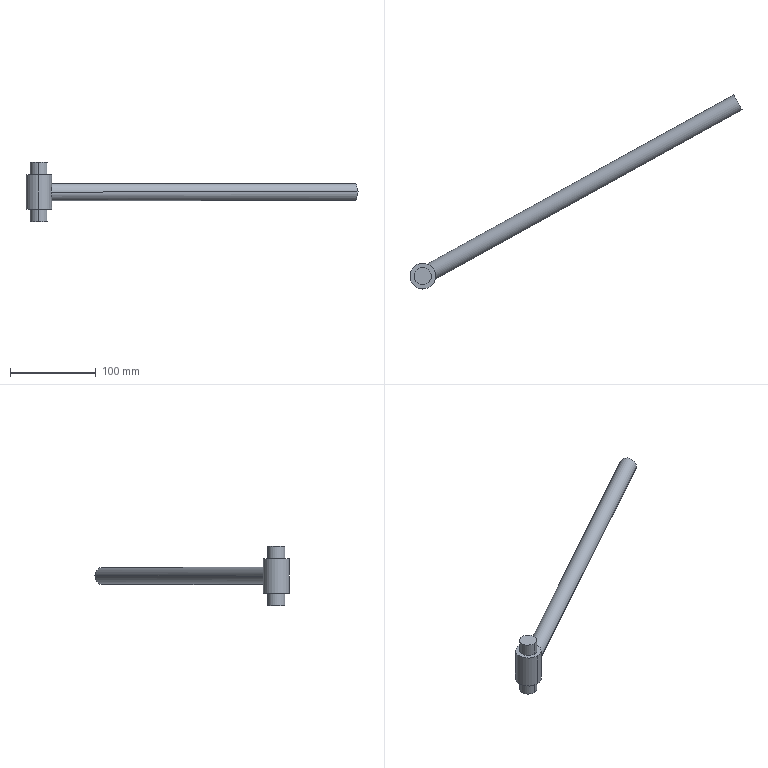Part | SolidWorks | 1 solid | 13 faces | box 387.638 x 226.527 x 70 mm | volume 165213 mm3 | cylinder 8 | plane 5 | commonest cylinder face diameters 20 x6 30 x2
STEP:
#1=CARTESIAN_POINT('',(1625.676,-816.887,527.206));
#2=VERTEX_POINT('',#1);
#3=CARTESIAN_POINT('',(1635.331,-834.402,527.206));
#4=VERTEX_POINT('',#3);
#5=CARTESIAN_POINT('',(1625.676,-816.887,527.206));
#6=CARTESIAN_POINT('',(1625.676,-816.887,527.892));
#7=CARTESIAN_POINT('',(1625.765,-816.918,528.559));
#8=CARTESIAN_POINT('',(1626.012,-817.009,529.536));
#9=CARTESIAN_POINT('',(1626.114,-817.048,529.859));
#10=CARTESIAN_POINT('',(1626.351,-817.142,530.492));
#11=CARTESIAN_POINT('',(1626.485,-817.197,530.799));
#12=CARTESIAN_POINT('',(1626.778,-817.323,531.395));
#13=CARTESIAN_POINT('',(1626.938,-817.394,531.685));
#14=CARTESIAN_POINT('',(1627.278,-817.554,532.248));
#15=CARTESIAN_POINT('',(1627.46,-817.644,532.523));
#16=CARTESIAN_POINT('',(1628.029,-817.941,533.317));
#17=CARTESIAN_POINT('',(1628.436,-818.173,533.804));
#18=CARTESIAN_POINT('',(1629.285,-818.723,534.702));
#19=CARTESIAN_POINT('',(1629.732,-819.044,535.115));
#20=CARTESIAN_POINT('',(1630.617,-819.763,535.834));
#21=CARTESIAN_POINT('',(1631.058,-820.163,536.144));
#22=CARTESIAN_POINT('',(1631.709,-820.836,536.53));
#23=CARTESIAN_POINT('',(1631.925,-821.074,536.646));
#24=CARTESIAN_POINT('',(1632.348,-821.57,536.847));
#25=CARTESIAN_POINT('',(1632.552,-821.826,536.931));
#26=CARTESIAN_POINT('',(1633.142,-822.62,537.134));
#27=CARTESIAN_POINT('',(1633.505,-823.181,537.204));
#28=CARTESIAN_POINT('',(1634.001,-824.076,537.207));
#29=CARTESIAN_POINT('',(1634.156,-824.381,537.19));
#30=CARTESIAN_POINT('',(1634.442,-824.991,537.123));
#31=CARTESIAN_POINT('',(1634.573,-825.299,537.073));
#32=CARTESIAN_POINT('',(1634.933,-826.225,536.873));
#33=CARTESIAN_POINT('',(1635.13,-826.856,536.671));
#34=CARTESIAN_POINT('',(1635.429,-828.074,536.158));
#35=CARTESIAN_POINT('',(1635.535,-828.669,535.845));
#36=CARTESIAN_POINT('',(1635.673,-829.817,535.118));
#37=CARTESIAN_POINT('',(1635.705,-830.357,534.712));
#38=CARTESIAN_POINT('',(1635.717,-831.372,533.814));
#39=CARTESIAN_POINT('',(1635.697,-831.849,533.318));
#40=CARTESIAN_POINT('',(1635.627,-832.696,532.266));
#41=CARTESIAN_POINT('',(1635.578,-833.07,531.708));
#42=CARTESIAN_POINT('',(1635.503,-833.545,530.814));
#43=CARTESIAN_POINT('',(1635.478,-833.689,530.504));
#44=CARTESIAN_POINT('',(1635.43,-833.941,529.871));
#45=CARTESIAN_POINT('',(1635.408,-834.048,529.55));
#46=CARTESIAN_POINT('',(1635.372,-834.222,528.897));
#47=CARTESIAN_POINT('',(1635.357,-834.289,528.565));
#48=CARTESIAN_POINT('',(1635.337,-834.379,527.89));
#49=CARTESIAN_POINT('',(1635.331,-834.402,527.546));
#50=CARTESIAN_POINT('',(1635.331,-834.402,527.206));
#51=B_SPLINE_CURVE_WITH_KNOTS('',3,(#5,#6,#7,#8,#9,#10,#11,#12,#13,#14,#15,#16,#17,#18,#19,#20,#21,#22,#23,#24,#25,#26,#27,#28,#29,#30,#31,#32,#33,#34,#35,#36,#37,#38,#39,#40,#41,#42,#43,#44,#45,#46,#47,#48,#49,#50),.UNSPECIFIED.,.F.,.F.,(4,2,2,2,2,2,2,2,2,2,2,2,2,2,2,2,2,2,2,2,2,2,4),(0.,0.002019,0.003028,0.004037,0.005047,0.006056,0.008075,0.01009,0.01211,0.01312,0.01413,0.01615,0.01716,0.01817,0.02019,0.02221,0.02422,0.02624,0.02826,0.02927,0.03028,0.03129,0.0323),.UNSPECIFIED.);
#52=EDGE_CURVE('',#2,#4,#51,.T.);
#53=ORIENTED_EDGE('',*,*,#52,.T.);
#54=CARTESIAN_POINT('',(1993.351,-637.03,527.206));
#55=VERTEX_POINT('',#54);
#56=CARTESIAN_POINT('',(1625.54,-839.8,527.206));
#57=DIRECTION('',(0.8757,0.4828,0.));
#58=VECTOR('',#57,1000.);
#59=LINE('',#56,#58);
#60=EDGE_CURVE('',#4,#55,#59,.T.);
#61=ORIENTED_EDGE('',*,*,#60,.T.);
#62=CARTESIAN_POINT('',(1983.695,-619.515,527.206));
#63=VERTEX_POINT('',#62);
#64=CARTESIAN_POINT('',(1988.523,-628.273,527.206));
#65=DIRECTION('',(0.8757,0.4828,0.));
#66=DIRECTION('',(-0.4828,0.8757,0.));
#67=AXIS2_PLACEMENT_3D('',#64,#65,#66);
#68=CIRCLE('',#67,10.);
#69=EDGE_CURVE('',#63,#55,#68,.T.);
#70=ORIENTED_EDGE('',*,*,#69,.F.);
#71=CARTESIAN_POINT('',(1615.885,-822.285,527.206));
#72=DIRECTION('',(0.8757,0.4828,0.));
#73=VECTOR('',#72,1000.);
#74=LINE('',#71,#73);
#75=EDGE_CURVE('',#2,#63,#74,.T.);
#76=ORIENTED_EDGE('',*,*,#75,.F.);
#77=EDGE_LOOP('',(#53,#61,#70,#76));
#78=FACE_OUTER_BOUND('',#77,.T.);
#79=CARTESIAN_POINT('',(1620.712,-831.042,527.206));
#80=DIRECTION('',(0.8757,0.4828,0.));
#81=DIRECTION('',(-0.4828,0.8757,0.));
#82=AXIS2_PLACEMENT_3D('',#79,#80,#81);
#83=CYLINDRICAL_SURFACE('',#82,10.);
#84=ADVANCED_FACE('',(#78),#83,.T.);
#85=CARTESIAN_POINT('',(1620.712,-821.042,547.206));
#86=VERTEX_POINT('',#85);
#87=CARTESIAN_POINT('',(1620.712,-841.042,547.206));
#88=VERTEX_POINT('',#87);
#89=CARTESIAN_POINT('',(1620.712,-831.042,547.206));
#90=DIRECTION('',(0.,0.,-1.));
#91=DIRECTION('',(0.,1.,0.));
#92=AXIS2_PLACEMENT_3D('',#89,#90,#91);
#93=CIRCLE('',#92,10.);
#94=EDGE_CURVE('',#86,#88,#93,.T.);
#95=ORIENTED_EDGE('',*,*,#94,.F.);
#96=CARTESIAN_POINT('',(1620.712,-821.042,562.206));
#97=VERTEX_POINT('',#96);
#98=CARTESIAN_POINT('',(1620.712,-821.042,492.206));
#99=DIRECTION('',(0.,0.,1.));
#100=VECTOR('',#99,1000.);
#101=LINE('',#98,#100);
#102=EDGE_CURVE('',#86,#97,#101,.T.);
#103=ORIENTED_EDGE('',*,*,#102,.T.);
#104=CARTESIAN_POINT('',(1620.712,-841.042,562.206));
#105=VERTEX_POINT('',#104);
#106=CARTESIAN_POINT('',(1620.712,-831.042,562.206));
#107=DIRECTION('',(0.,0.,-1.));
#108=DIRECTION('',(0.,1.,0.));
#109=AXIS2_PLACEMENT_3D('',#106,#107,#108);
#110=CIRCLE('',#109,10.);
#111=EDGE_CURVE('',#97,#105,#110,.T.);
#112=ORIENTED_EDGE('',*,*,#111,.T.);
#113=CARTESIAN_POINT('',(1620.712,-841.042,492.206));
#114=DIRECTION('',(0.,0.,1.));
#115=VECTOR('',#114,1000.);
#116=LINE('',#113,#115);
#117=EDGE_CURVE('',#88,#105,#116,.T.);
#118=ORIENTED_EDGE('',*,*,#117,.F.);
#119=EDGE_LOOP('',(#95,#103,#112,#118));
#120=FACE_OUTER_BOUND('',#119,.T.);
#121=CARTESIAN_POINT('',(1620.712,-831.042,492.206));
#122=DIRECTION('',(0.,0.,1.));
#123=DIRECTION('',(0.,-1.,0.));
#124=AXIS2_PLACEMENT_3D('',#121,#122,#123);
#125=CYLINDRICAL_SURFACE('',#124,10.);
#126=ADVANCED_FACE('',(#120),#125,.T.);
#127=ORIENTED_EDGE('',*,*,#52,.F.);
#128=CARTESIAN_POINT('',(1635.331,-834.402,527.206));
#129=CARTESIAN_POINT('',(1635.331,-834.402,526.529));
#130=CARTESIAN_POINT('',(1635.353,-834.312,525.862));
#131=CARTESIAN_POINT('',(1635.426,-833.964,524.543));
#132=CARTESIAN_POINT('',(1635.477,-833.711,523.915));
#133=CARTESIAN_POINT('',(1635.552,-833.237,523.018));
#134=CARTESIAN_POINT('',(1635.577,-833.062,522.724));
#135=CARTESIAN_POINT('',(1635.623,-832.687,522.159));
#136=CARTESIAN_POINT('',(1635.644,-832.487,521.887));
#137=CARTESIAN_POINT('',(1635.679,-832.063,521.361));
#138=CARTESIAN_POINT('',(1635.693,-831.84,521.107));
#139=CARTESIAN_POINT('',(1635.711,-831.371,520.618));
#140=CARTESIAN_POINT('',(1635.714,-831.125,520.38));
#141=CARTESIAN_POINT('',(1635.706,-830.363,519.705));
#142=CARTESIAN_POINT('',(1635.674,-829.825,519.301));
#143=CARTESIAN_POINT('',(1635.572,-828.977,518.762));
#144=CARTESIAN_POINT('',(1635.53,-828.687,518.593));
#145=CARTESIAN_POINT('',(1635.423,-828.094,518.28));
#146=CARTESIAN_POINT('',(1635.359,-827.789,518.136));
#147=CARTESIAN_POINT('',(1635.136,-826.877,517.749));
#148=CARTESIAN_POINT('',(1634.946,-826.261,517.55));
#149=CARTESIAN_POINT('',(1634.585,-825.328,517.345));
#150=CARTESIAN_POINT('',(1634.453,-825.016,517.293));
#151=CARTESIAN_POINT('',(1634.169,-824.406,517.224));
#152=CARTESIAN_POINT('',(1634.016,-824.106,517.207));
#153=CARTESIAN_POINT('',(1633.692,-823.516,517.206));
#154=CARTESIAN_POINT('',(1633.519,-823.226,517.222));
#155=CARTESIAN_POINT('',(1633.154,-822.656,517.29));
#156=CARTESIAN_POINT('',(1632.961,-822.377,517.342));
#157=CARTESIAN_POINT('',(1632.368,-821.576,517.544));
#158=CARTESIAN_POINT('',(1631.948,-821.084,517.742));
#159=CARTESIAN_POINT('',(1631.071,-820.175,518.26));
#160=CARTESIAN_POINT('',(1630.625,-819.77,518.572));
#161=CARTESIAN_POINT('',(1629.736,-819.047,519.294));
#162=CARTESIAN_POINT('',(1629.29,-818.726,519.707));
#163=CARTESIAN_POINT('',(1628.439,-818.176,520.604));
#164=CARTESIAN_POINT('',(1628.033,-817.943,521.09));
#165=CARTESIAN_POINT('',(1627.465,-817.646,521.883));
#166=CARTESIAN_POINT('',(1627.282,-817.556,522.159));
#167=CARTESIAN_POINT('',(1626.941,-817.395,522.722));
#168=CARTESIAN_POINT('',(1626.782,-817.324,523.012));
#169=CARTESIAN_POINT('',(1626.489,-817.198,523.606));
#170=CARTESIAN_POINT('',(1626.355,-817.143,523.912));
#171=CARTESIAN_POINT('',(1626.119,-817.05,524.541));
#172=CARTESIAN_POINT('',(1626.015,-817.01,524.866));
#173=CARTESIAN_POINT('',(1625.848,-816.949,525.523));
#174=CARTESIAN_POINT('',(1625.784,-816.926,525.854));
#175=CARTESIAN_POINT('',(1625.698,-816.895,526.525));
#176=CARTESIAN_POINT('',(1625.676,-816.887,526.865));
#177=CARTESIAN_POINT('',(1625.676,-816.887,527.206));
#178=B_SPLINE_CURVE_WITH_KNOTS('',3,(#128,#129,#130,#131,#132,#133,#134,#135,#136,#137,#138,#139,#140,#141,#142,#143,#144,#145,#146,#147,#148,#149,#150,#151,#152,#153,#154,#155,#156,#157,#158,#159,#160,#161,#162,#163,#164,#165,#166,#167,#168,#169,#170,#171,#172,#173,#174,#175,#176,#177),.UNSPECIFIED.,.F.,.F.,(4,2,2,2,2,2,2,2,2,2,2,2,2,2,2,2,2,2,2,2,2,2,2,2,4),(0.0323,0.03431,0.03632,0.03733,0.03834,0.03934,0.04035,0.04236,0.04337,0.04437,0.04639,0.04739,0.0484,0.04941,0.05041,0.05242,0.05444,0.05645,0.05846,0.05947,0.06048,0.06148,0.06249,0.06349,0.0645),.UNSPECIFIED.);
#179=EDGE_CURVE('',#4,#2,#178,.T.);
#180=ORIENTED_EDGE('',*,*,#179,.F.);
#181=EDGE_LOOP('',(#127,#180));
#182=FACE_BOUND('',#181,.T.);
#183=CARTESIAN_POINT('',(1620.712,-816.042,507.206));
#184=VERTEX_POINT('',#183);
#185=CARTESIAN_POINT('',(1620.712,-846.042,507.206));
#186=VERTEX_POINT('',#185);
#187=CARTESIAN_POINT('',(1620.712,-831.042,507.206));
#188=DIRECTION('',(0.,0.,-1.));
#189=DIRECTION('',(0.,1.,0.));
#190=AXIS2_PLACEMENT_3D('',#187,#188,#189);
#191=CIRCLE('',#190,15.);
#192=EDGE_CURVE('',#184,#186,#191,.T.);
#193=ORIENTED_EDGE('',*,*,#192,.F.);
#194=CARTESIAN_POINT('',(1620.712,-816.042,547.206));
#195=VERTEX_POINT('',#194);
#196=CARTESIAN_POINT('',(1620.712,-816.042,507.206));
#197=DIRECTION('',(0.,0.,1.));
#198=VECTOR('',#197,1000.);
#199=LINE('',#196,#198);
#200=EDGE_CURVE('',#184,#195,#199,.T.);
#201=ORIENTED_EDGE('',*,*,#200,.T.);
#202=CARTESIAN_POINT('',(1620.712,-846.042,547.206));
#203=VERTEX_POINT('',#202);
#204=CARTESIAN_POINT('',(1620.712,-831.042,547.206));
#205=DIRECTION('',(0.,0.,-1.));
#206=DIRECTION('',(0.,1.,0.));
#207=AXIS2_PLACEMENT_3D('',#204,#205,#206);
#208=CIRCLE('',#207,15.);
#209=EDGE_CURVE('',#195,#203,#208,.T.);
#210=ORIENTED_EDGE('',*,*,#209,.T.);
#211=CARTESIAN_POINT('',(1620.712,-846.042,507.206));
#212=DIRECTION('',(0.,0.,1.));
#213=VECTOR('',#212,1000.);
#214=LINE('',#211,#213);
#215=EDGE_CURVE('',#186,#203,#214,.T.);
#216=ORIENTED_EDGE('',*,*,#215,.F.);
#217=EDGE_LOOP('',(#193,#201,#210,#216));
#218=FACE_OUTER_BOUND('',#217,.T.);
#219=CARTESIAN_POINT('',(1620.712,-831.042,507.206));
#220=DIRECTION('',(0.,0.,1.));
#221=DIRECTION('',(0.,-1.,0.));
#222=AXIS2_PLACEMENT_3D('',#219,#220,#221);
#223=CYLINDRICAL_SURFACE('',#222,15.);
#224=ADVANCED_FACE('',(#182,#218),#223,.T.);
#225=CARTESIAN_POINT('',(1620.712,-821.042,492.206));
#226=VERTEX_POINT('',#225);
#227=CARTESIAN_POINT('',(1620.712,-841.042,492.206));
#228=VERTEX_POINT('',#227);
#229=CARTESIAN_POINT('',(1620.712,-831.042,492.206));
#230=DIRECTION('',(0.,0.,-1.));
#231=DIRECTION('',(0.,1.,0.));
#232=AXIS2_PLACEMENT_3D('',#229,#230,#231);
#233=CIRCLE('',#232,10.);
#234=EDGE_CURVE('',#226,#228,#233,.T.);
#235=ORIENTED_EDGE('',*,*,#234,.F.);
#236=CARTESIAN_POINT('',(1620.712,-821.042,507.206));
#237=VERTEX_POINT('',#236);
#238=CARTESIAN_POINT('',(1620.712,-821.042,492.206));
#239=DIRECTION('',(0.,0.,1.));
#240=VECTOR('',#239,1000.);
#241=LINE('',#238,#240);
#242=EDGE_CURVE('',#226,#237,#241,.T.);
#243=ORIENTED_EDGE('',*,*,#242,.T.);
#244=CARTESIAN_POINT('',(1620.712,-841.042,507.206));
#245=VERTEX_POINT('',#244);
#246=CARTESIAN_POINT('',(1620.712,-831.042,507.206));
#247=DIRECTION('',(0.,0.,-1.));
#248=DIRECTION('',(0.,1.,0.));
#249=AXIS2_PLACEMENT_3D('',#246,#247,#248);
#250=CIRCLE('',#249,10.);
#251=EDGE_CURVE('',#237,#245,#250,.T.);
#252=ORIENTED_EDGE('',*,*,#251,.T.);
#253=CARTESIAN_POINT('',(1620.712,-841.042,492.206));
#254=DIRECTION('',(0.,0.,1.));
#255=VECTOR('',#254,1000.);
#256=LINE('',#253,#255);
#257=EDGE_CURVE('',#228,#245,#256,.T.);
#258=ORIENTED_EDGE('',*,*,#257,.F.);
#259=EDGE_LOOP('',(#235,#243,#252,#258));
#260=FACE_OUTER_BOUND('',#259,.T.);
#261=CARTESIAN_POINT('',(1620.712,-831.042,492.206));
#262=DIRECTION('',(0.,0.,1.));
#263=DIRECTION('',(0.,-1.,0.));
#264=AXIS2_PLACEMENT_3D('',#261,#262,#263);
#265=CYLINDRICAL_SURFACE('',#264,10.);
#266=ADVANCED_FACE('',(#260),#265,.T.);
#267=ORIENTED_EDGE('',*,*,#242,.F.);
#268=CARTESIAN_POINT('',(1620.712,-831.042,492.206));
#269=DIRECTION('',(0.,0.,-1.));
#270=DIRECTION('',(0.,1.,0.));
#271=AXIS2_PLACEMENT_3D('',#268,#269,#270);
#272=CIRCLE('',#271,10.);
#273=EDGE_CURVE('',#228,#226,#272,.T.);
#274=ORIENTED_EDGE('',*,*,#273,.F.);
#275=ORIENTED_EDGE('',*,*,#257,.T.);
#276=CARTESIAN_POINT('',(1620.712,-831.042,507.206));
#277=DIRECTION('',(0.,0.,-1.));
#278=DIRECTION('',(0.,1.,0.));
#279=AXIS2_PLACEMENT_3D('',#276,#277,#278);
#280=CIRCLE('',#279,10.);
#281=EDGE_CURVE('',#245,#237,#280,.T.);
#282=ORIENTED_EDGE('',*,*,#281,.T.);
#283=EDGE_LOOP('',(#267,#274,#275,#282));
#284=FACE_OUTER_BOUND('',#283,.T.);
#285=CARTESIAN_POINT('',(1620.712,-831.042,492.206));
#286=DIRECTION('',(0.,0.,1.));
#287=DIRECTION('',(0.,-1.,0.));
#288=AXIS2_PLACEMENT_3D('',#285,#286,#287);
#289=CYLINDRICAL_SURFACE('',#288,10.);
#290=ADVANCED_FACE('',(#284),#289,.T.);
#291=ORIENTED_EDGE('',*,*,#273,.T.);
#292=ORIENTED_EDGE('',*,*,#234,.T.);
#293=EDGE_LOOP('',(#291,#292));
#294=FACE_OUTER_BOUND('',#293,.T.);
#295=CARTESIAN_POINT('',(1620.712,-831.042,492.206));
#296=DIRECTION('',(0.,0.,-1.));
#297=DIRECTION('',(0.,1.,0.));
#298=AXIS2_PLACEMENT_3D('',#295,#296,#297);
#299=PLANE('',#298);
#300=ADVANCED_FACE('',(#294),#299,.T.);
#301=ORIENTED_EDGE('',*,*,#200,.F.);
#302=CARTESIAN_POINT('',(1620.712,-831.042,507.206));
#303=DIRECTION('',(0.,0.,-1.));
#304=DIRECTION('',(0.,1.,0.));
#305=AXIS2_PLACEMENT_3D('',#302,#303,#304);
#306=CIRCLE('',#305,15.);
#307=EDGE_CURVE('',#186,#184,#306,.T.);
#308=ORIENTED_EDGE('',*,*,#307,.F.);
#309=ORIENTED_EDGE('',*,*,#215,.T.);
#310=CARTESIAN_POINT('',(1620.712,-831.042,547.206));
#311=DIRECTION('',(0.,0.,-1.));
#312=DIRECTION('',(0.,1.,0.));
#313=AXIS2_PLACEMENT_3D('',#310,#311,#312);
#314=CIRCLE('',#313,15.);
#315=EDGE_CURVE('',#203,#195,#314,.T.);
#316=ORIENTED_EDGE('',*,*,#315,.T.);
#317=EDGE_LOOP('',(#301,#308,#309,#316));
#318=FACE_OUTER_BOUND('',#317,.T.);
#319=CARTESIAN_POINT('',(1620.712,-831.042,507.206));
#320=DIRECTION('',(0.,0.,1.));
#321=DIRECTION('',(0.,-1.,0.));
#322=AXIS2_PLACEMENT_3D('',#319,#320,#321);
#323=CYLINDRICAL_SURFACE('',#322,15.);
#324=ADVANCED_FACE('',(#318),#323,.T.);
#325=ORIENTED_EDGE('',*,*,#281,.F.);
#326=ORIENTED_EDGE('',*,*,#251,.F.);
#327=EDGE_LOOP('',(#325,#326));
#328=FACE_BOUND('',#327,.T.);
#329=ORIENTED_EDGE('',*,*,#307,.T.);
#330=ORIENTED_EDGE('',*,*,#192,.T.);
#331=EDGE_LOOP('',(#329,#330));
#332=FACE_OUTER_BOUND('',#331,.T.);
#333=CARTESIAN_POINT('',(1620.712,-831.042,507.206));
#334=DIRECTION('',(0.,0.,-1.));
#335=DIRECTION('',(0.,1.,0.));
#336=AXIS2_PLACEMENT_3D('',#333,#334,#335);
#337=PLANE('',#336);
#338=ADVANCED_FACE('',(#328,#332),#337,.T.);
#339=CARTESIAN_POINT('',(1620.712,-831.042,547.206));
#340=DIRECTION('',(0.,0.,-1.));
#341=DIRECTION('',(0.,1.,0.));
#342=AXIS2_PLACEMENT_3D('',#339,#340,#341);
#343=CIRCLE('',#342,10.);
#344=EDGE_CURVE('',#88,#86,#343,.T.);
#345=ORIENTED_EDGE('',*,*,#344,.T.);
#346=ORIENTED_EDGE('',*,*,#94,.T.);
#347=EDGE_LOOP('',(#345,#346));
#348=FACE_BOUND('',#347,.T.);
#349=ORIENTED_EDGE('',*,*,#315,.F.);
#350=ORIENTED_EDGE('',*,*,#209,.F.);
#351=EDGE_LOOP('',(#349,#350));
#352=FACE_OUTER_BOUND('',#351,.T.);
#353=CARTESIAN_POINT('',(1620.712,-831.042,547.206));
#354=DIRECTION('',(0.,0.,-1.));
#355=DIRECTION('',(0.,1.,0.));
#356=AXIS2_PLACEMENT_3D('',#353,#354,#355);
#357=PLANE('',#356);
#358=ADVANCED_FACE('',(#348,#352),#357,.F.);
#359=CARTESIAN_POINT('',(1620.712,-831.042,562.206));
#360=DIRECTION('',(0.,0.,-1.));
#361=DIRECTION('',(0.,1.,0.));
#362=AXIS2_PLACEMENT_3D('',#359,#360,#361);
#363=CIRCLE('',#362,10.);
#364=EDGE_CURVE('',#105,#97,#363,.T.);
#365=ORIENTED_EDGE('',*,*,#364,.F.);
#366=ORIENTED_EDGE('',*,*,#111,.F.);
#367=EDGE_LOOP('',(#365,#366));
#368=FACE_OUTER_BOUND('',#367,.T.);
#369=CARTESIAN_POINT('',(1620.712,-831.042,562.206));
#370=DIRECTION('',(0.,0.,-1.));
#371=DIRECTION('',(0.,1.,0.));
#372=AXIS2_PLACEMENT_3D('',#369,#370,#371);
#373=PLANE('',#372);
#374=ADVANCED_FACE('',(#368),#373,.F.);
#375=ORIENTED_EDGE('',*,*,#102,.F.);
#376=ORIENTED_EDGE('',*,*,#344,.F.);
#377=ORIENTED_EDGE('',*,*,#117,.T.);
#378=ORIENTED_EDGE('',*,*,#364,.T.);
#379=EDGE_LOOP('',(#375,#376,#377,#378));
#380=FACE_OUTER_BOUND('',#379,.T.);
#381=CARTESIAN_POINT('',(1620.712,-831.042,492.206));
#382=DIRECTION('',(0.,0.,1.));
#383=DIRECTION('',(0.,-1.,0.));
#384=AXIS2_PLACEMENT_3D('',#381,#382,#383);
#385=CYLINDRICAL_SURFACE('',#384,10.);
#386=ADVANCED_FACE('',(#380),#385,.T.);
#387=ORIENTED_EDGE('',*,*,#69,.T.);
#388=CARTESIAN_POINT('',(1988.523,-628.273,527.206));
#389=DIRECTION('',(0.8757,0.4828,0.));
#390=DIRECTION('',(-0.4828,0.8757,0.));
#391=AXIS2_PLACEMENT_3D('',#388,#389,#390);
#392=CIRCLE('',#391,10.);
#393=EDGE_CURVE('',#55,#63,#392,.T.);
#394=ORIENTED_EDGE('',*,*,#393,.T.);
#395=EDGE_LOOP('',(#387,#394));
#396=FACE_OUTER_BOUND('',#395,.T.);
#397=CARTESIAN_POINT('',(1988.523,-628.273,527.206));
#398=DIRECTION('',(0.8757,0.4828,0.));
#399=DIRECTION('',(-0.4828,0.8757,0.));
#400=AXIS2_PLACEMENT_3D('',#397,#398,#399);
#401=PLANE('',#400);
#402=ADVANCED_FACE('',(#396),#401,.T.);
#403=ORIENTED_EDGE('',*,*,#60,.F.);
#404=ORIENTED_EDGE('',*,*,#179,.T.);
#405=ORIENTED_EDGE('',*,*,#75,.T.);
#406=ORIENTED_EDGE('',*,*,#393,.F.);
#407=EDGE_LOOP('',(#403,#404,#405,#406));
#408=FACE_OUTER_BOUND('',#407,.T.);
#409=CARTESIAN_POINT('',(1620.712,-831.042,527.206));
#410=DIRECTION('',(0.8757,0.4828,0.));
#411=DIRECTION('',(-0.4828,0.8757,0.));
#412=AXIS2_PLACEMENT_3D('',#409,#410,#411);
#413=CYLINDRICAL_SURFACE('',#412,10.);
#414=ADVANCED_FACE('',(#408),#413,.T.);
#415=CLOSED_SHELL('',(#84,#126,#224,#266,#290,#300,#324,#338,#358,#374,#386,#402,#414));
#416=MANIFOLD_SOLID_BREP('',#415);
#417=CARTESIAN_POINT('',(0.,0.,0.));
#418=DIRECTION('',(0.,0.,1.));
#419=DIRECTION('',(1.,0.,0.));
#420=AXIS2_PLACEMENT_3D('',#417,#418,#419);
#421=(LENGTH_UNIT()NAMED_UNIT(*)SI_UNIT(.MILLI.,.METRE.));
#422=UNCERTAINTY_MEASURE_WITH_UNIT(LENGTH_MEASURE(0.00001),#421,'','');
#423=(NAMED_UNIT(*)PLANE_ANGLE_UNIT()SI_UNIT($,.RADIAN.));
#424=(NAMED_UNIT(*)SI_UNIT($,.STERADIAN.)SOLID_ANGLE_UNIT());
#425=(GEOMETRIC_REPRESENTATION_CONTEXT(3)GLOBAL_UNCERTAINTY_ASSIGNED_CONTEXT((#422))GLOBAL_UNIT_ASSIGNED_CONTEXT((#421,#423,#424))REPRESENTATION_CONTEXT('',''));
#426=ADVANCED_BREP_SHAPE_REPRESENTATION('',(#416,#420),#425);